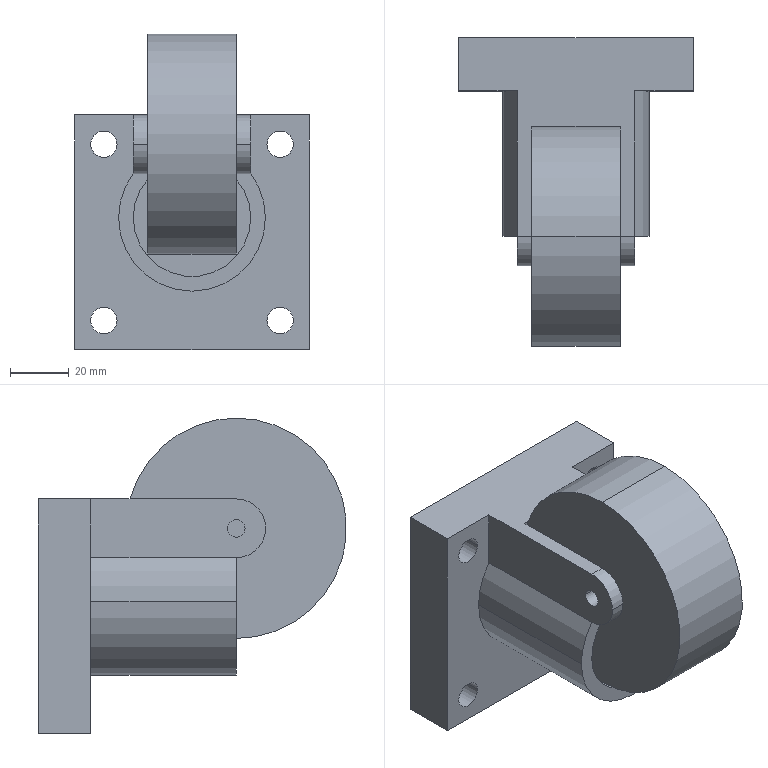Part | NX | 1 solid | 42 faces | box 80 x 105 x 107.5 mm | volume 301062 mm3 | cylinder 24 | plane 18 | commonest cylinder face diameters 9 x8 6 x4 20 x4 40 x3 50 x3 75 x2
STEP:
#1=CARTESIAN_POINT('',(-40.,4.5,0.));
#2=VERTEX_POINT('',#1);
#3=CARTESIAN_POINT('',(-40.,22.5,0.));
#4=VERTEX_POINT('',#3);
#5=CARTESIAN_POINT('',(-40.,0.,0.));
#6=DIRECTION('',(0.,1.,0.));
#7=VECTOR('',#6,1000.);
#8=LINE('',#5,#7);
#9=EDGE_CURVE('',#2,#4,#8,.T.);
#10=ORIENTED_EDGE('',*,*,#9,.T.);
#11=CARTESIAN_POINT('',(40.,22.5,0.));
#12=VERTEX_POINT('',#11);
#13=CARTESIAN_POINT('',(0.,22.5,0.));
#14=DIRECTION('',(-1.,0.,0.));
#15=VECTOR('',#14,1000.);
#16=LINE('',#13,#15);
#17=EDGE_CURVE('',#12,#4,#16,.T.);
#18=ORIENTED_EDGE('',*,*,#17,.F.);
#19=CARTESIAN_POINT('',(40.,4.5,0.));
#20=VERTEX_POINT('',#19);
#21=CARTESIAN_POINT('',(40.,0.,0.));
#22=DIRECTION('',(0.,-1.,0.));
#23=VECTOR('',#22,1000.);
#24=LINE('',#21,#23);
#25=EDGE_CURVE('',#12,#20,#24,.T.);
#26=ORIENTED_EDGE('',*,*,#25,.T.);
#27=CARTESIAN_POINT('',(0.,4.5,0.));
#28=DIRECTION('',(1.,0.,0.));
#29=VECTOR('',#28,1000.);
#30=LINE('',#27,#29);
#31=EDGE_CURVE('',#2,#20,#30,.T.);
#32=ORIENTED_EDGE('',*,*,#31,.F.);
#33=EDGE_LOOP('',(#10,#18,#26,#32));
#34=FACE_BOUND('',#33,.T.);
#35=CARTESIAN_POINT('',(0.,0.,0.));
#36=DIRECTION('',(0.,0.,1.));
#37=DIRECTION('',(1.,0.,0.));
#38=AXIS2_PLACEMENT_3D('',#35,#36,#37);
#39=PLANE('',#38);
#40=ADVANCED_FACE('',(#34),#39,.F.);
#41=ORIENTED_EDGE('',*,*,#9,.F.);
#42=CARTESIAN_POINT('',(-40.,4.5,80.));
#43=VERTEX_POINT('',#42);
#44=CARTESIAN_POINT('',(-40.,4.5,0.));
#45=DIRECTION('',(0.,0.,1.));
#46=VECTOR('',#45,1000.);
#47=LINE('',#44,#46);
#48=EDGE_CURVE('',#2,#43,#47,.T.);
#49=ORIENTED_EDGE('',*,*,#48,.T.);
#50=CARTESIAN_POINT('',(-40.,22.5,80.));
#51=VERTEX_POINT('',#50);
#52=CARTESIAN_POINT('',(-40.,0.,80.));
#53=DIRECTION('',(0.,1.,0.));
#54=VECTOR('',#53,1000.);
#55=LINE('',#52,#54);
#56=EDGE_CURVE('',#43,#51,#55,.T.);
#57=ORIENTED_EDGE('',*,*,#56,.T.);
#58=CARTESIAN_POINT('',(-40.,22.5,0.));
#59=DIRECTION('',(0.,0.,-1.));
#60=VECTOR('',#59,1000.);
#61=LINE('',#58,#60);
#62=EDGE_CURVE('',#51,#4,#61,.T.);
#63=ORIENTED_EDGE('',*,*,#62,.T.);
#64=EDGE_LOOP('',(#41,#49,#57,#63));
#65=FACE_BOUND('',#64,.T.);
#66=CARTESIAN_POINT('',(-40.,7.5,0.));
#67=DIRECTION('',(-1.,0.,0.));
#68=DIRECTION('',(0.,0.,1.));
#69=AXIS2_PLACEMENT_3D('',#66,#67,#68);
#70=PLANE('',#69);
#71=ADVANCED_FACE('',(#65),#70,.T.);
#72=ORIENTED_EDGE('',*,*,#17,.T.);
#73=ORIENTED_EDGE('',*,*,#62,.F.);
#74=CARTESIAN_POINT('',(40.,22.5,80.));
#75=VERTEX_POINT('',#74);
#76=CARTESIAN_POINT('',(0.,22.5,80.));
#77=DIRECTION('',(-1.,0.,0.));
#78=VECTOR('',#77,1000.);
#79=LINE('',#76,#78);
#80=EDGE_CURVE('',#75,#51,#79,.T.);
#81=ORIENTED_EDGE('',*,*,#80,.F.);
#82=CARTESIAN_POINT('',(40.,22.5,0.));
#83=DIRECTION('',(0.,0.,1.));
#84=VECTOR('',#83,1000.);
#85=LINE('',#82,#84);
#86=EDGE_CURVE('',#12,#75,#85,.T.);
#87=ORIENTED_EDGE('',*,*,#86,.F.);
#88=EDGE_LOOP('',(#72,#73,#81,#87));
#89=FACE_BOUND('',#88,.T.);
#90=CARTESIAN_POINT('',(25.5,22.5,10.));
#91=VERTEX_POINT('',#90);
#92=CARTESIAN_POINT('',(34.5,22.5,10.));
#93=VERTEX_POINT('',#92);
#94=CARTESIAN_POINT('',(30.,22.5,10.));
#95=DIRECTION('',(0.,-1.,0.));
#96=DIRECTION('',(1.,0.,0.));
#97=AXIS2_PLACEMENT_3D('',#94,#95,#96);
#98=CIRCLE('',#97,4.5);
#99=EDGE_CURVE('',#91,#93,#98,.T.);
#100=ORIENTED_EDGE('',*,*,#99,.T.);
#101=CARTESIAN_POINT('',(30.,22.5,10.));
#102=DIRECTION('',(0.,-1.,0.));
#103=DIRECTION('',(1.,0.,0.));
#104=AXIS2_PLACEMENT_3D('',#101,#102,#103);
#105=CIRCLE('',#104,4.5);
#106=EDGE_CURVE('',#93,#91,#105,.T.);
#107=ORIENTED_EDGE('',*,*,#106,.T.);
#108=EDGE_LOOP('',(#100,#107));
#109=FACE_BOUND('',#108,.T.);
#110=CARTESIAN_POINT('',(-34.5,22.5,10.));
#111=VERTEX_POINT('',#110);
#112=CARTESIAN_POINT('',(-25.5,22.5,10.));
#113=VERTEX_POINT('',#112);
#114=CARTESIAN_POINT('',(-30.,22.5,10.));
#115=DIRECTION('',(0.,-1.,0.));
#116=DIRECTION('',(1.,0.,0.));
#117=AXIS2_PLACEMENT_3D('',#114,#115,#116);
#118=CIRCLE('',#117,4.5);
#119=EDGE_CURVE('',#111,#113,#118,.T.);
#120=ORIENTED_EDGE('',*,*,#119,.T.);
#121=CARTESIAN_POINT('',(-30.,22.5,10.));
#122=DIRECTION('',(0.,-1.,0.));
#123=DIRECTION('',(1.,0.,0.));
#124=AXIS2_PLACEMENT_3D('',#121,#122,#123);
#125=CIRCLE('',#124,4.5);
#126=EDGE_CURVE('',#113,#111,#125,.T.);
#127=ORIENTED_EDGE('',*,*,#126,.T.);
#128=EDGE_LOOP('',(#120,#127));
#129=FACE_BOUND('',#128,.T.);
#130=CARTESIAN_POINT('',(25.5,22.5,70.));
#131=VERTEX_POINT('',#130);
#132=CARTESIAN_POINT('',(34.5,22.5,70.));
#133=VERTEX_POINT('',#132);
#134=CARTESIAN_POINT('',(30.,22.5,70.));
#135=DIRECTION('',(0.,-1.,0.));
#136=DIRECTION('',(1.,0.,0.));
#137=AXIS2_PLACEMENT_3D('',#134,#135,#136);
#138=CIRCLE('',#137,4.5);
#139=EDGE_CURVE('',#131,#133,#138,.T.);
#140=ORIENTED_EDGE('',*,*,#139,.T.);
#141=CARTESIAN_POINT('',(30.,22.5,70.));
#142=DIRECTION('',(0.,-1.,0.));
#143=DIRECTION('',(1.,0.,0.));
#144=AXIS2_PLACEMENT_3D('',#141,#142,#143);
#145=CIRCLE('',#144,4.5);
#146=EDGE_CURVE('',#133,#131,#145,.T.);
#147=ORIENTED_EDGE('',*,*,#146,.T.);
#148=EDGE_LOOP('',(#140,#147));
#149=FACE_BOUND('',#148,.T.);
#150=CARTESIAN_POINT('',(-34.5,22.5,70.));
#151=VERTEX_POINT('',#150);
#152=CARTESIAN_POINT('',(-25.5,22.5,70.));
#153=VERTEX_POINT('',#152);
#154=CARTESIAN_POINT('',(-30.,22.5,70.));
#155=DIRECTION('',(0.,-1.,0.));
#156=DIRECTION('',(1.,0.,0.));
#157=AXIS2_PLACEMENT_3D('',#154,#155,#156);
#158=CIRCLE('',#157,4.5);
#159=EDGE_CURVE('',#151,#153,#158,.T.);
#160=ORIENTED_EDGE('',*,*,#159,.T.);
#161=CARTESIAN_POINT('',(-30.,22.5,70.));
#162=DIRECTION('',(0.,-1.,0.));
#163=DIRECTION('',(1.,0.,0.));
#164=AXIS2_PLACEMENT_3D('',#161,#162,#163);
#165=CIRCLE('',#164,4.5);
#166=EDGE_CURVE('',#153,#151,#165,.T.);
#167=ORIENTED_EDGE('',*,*,#166,.T.);
#168=EDGE_LOOP('',(#160,#167));
#169=FACE_BOUND('',#168,.T.);
#170=CARTESIAN_POINT('',(40.,22.5,0.));
#171=DIRECTION('',(0.,1.,0.));
#172=DIRECTION('',(1.,0.,0.));
#173=AXIS2_PLACEMENT_3D('',#170,#171,#172);
#174=PLANE('',#173);
#175=ADVANCED_FACE('',(#89,#109,#129,#149,#169),#174,.T.);
#176=ORIENTED_EDGE('',*,*,#25,.F.);
#177=ORIENTED_EDGE('',*,*,#86,.T.);
#178=CARTESIAN_POINT('',(40.,4.5,80.));
#179=VERTEX_POINT('',#178);
#180=CARTESIAN_POINT('',(40.,0.,80.));
#181=DIRECTION('',(0.,-1.,0.));
#182=VECTOR('',#181,1000.);
#183=LINE('',#180,#182);
#184=EDGE_CURVE('',#75,#179,#183,.T.);
#185=ORIENTED_EDGE('',*,*,#184,.T.);
#186=CARTESIAN_POINT('',(40.,4.5,0.));
#187=DIRECTION('',(0.,0.,-1.));
#188=VECTOR('',#187,1000.);
#189=LINE('',#186,#188);
#190=EDGE_CURVE('',#179,#20,#189,.T.);
#191=ORIENTED_EDGE('',*,*,#190,.T.);
#192=EDGE_LOOP('',(#176,#177,#185,#191));
#193=FACE_BOUND('',#192,.T.);
#194=CARTESIAN_POINT('',(40.,-7.5,0.));
#195=DIRECTION('',(1.,0.,0.));
#196=DIRECTION('',(0.,1.,0.));
#197=AXIS2_PLACEMENT_3D('',#194,#195,#196);
#198=PLANE('',#197);
#199=ADVANCED_FACE('',(#193),#198,.T.);
#200=CARTESIAN_POINT('',(-20.,4.5,60.));
#201=VERTEX_POINT('',#200);
#202=CARTESIAN_POINT('',(-25.,4.5,45.));
#203=VERTEX_POINT('',#202);
#204=CARTESIAN_POINT('',(0.,4.5,45.));
#205=DIRECTION('',(0.,-1.,0.));
#206=DIRECTION('',(-1.,0.,0.));
#207=AXIS2_PLACEMENT_3D('',#204,#205,#206);
#208=CIRCLE('',#207,25.);
#209=EDGE_CURVE('',#201,#203,#208,.T.);
#210=ORIENTED_EDGE('',*,*,#209,.F.);
#211=CARTESIAN_POINT('',(-20.,4.5,80.));
#212=VERTEX_POINT('',#211);
#213=CARTESIAN_POINT('',(-20.,4.5,0.));
#214=DIRECTION('',(0.,0.,1.));
#215=VECTOR('',#214,1000.);
#216=LINE('',#213,#215);
#217=EDGE_CURVE('',#201,#212,#216,.T.);
#218=ORIENTED_EDGE('',*,*,#217,.T.);
#219=CARTESIAN_POINT('',(0.,4.5,80.));
#220=DIRECTION('',(1.,0.,0.));
#221=VECTOR('',#220,1000.);
#222=LINE('',#219,#221);
#223=EDGE_CURVE('',#43,#212,#222,.T.);
#224=ORIENTED_EDGE('',*,*,#223,.F.);
#225=ORIENTED_EDGE('',*,*,#48,.F.);
#226=ORIENTED_EDGE('',*,*,#31,.T.);
#227=ORIENTED_EDGE('',*,*,#190,.F.);
#228=CARTESIAN_POINT('',(20.,4.5,80.));
#229=VERTEX_POINT('',#228);
#230=CARTESIAN_POINT('',(0.,4.5,80.));
#231=DIRECTION('',(1.,0.,0.));
#232=VECTOR('',#231,1000.);
#233=LINE('',#230,#232);
#234=EDGE_CURVE('',#229,#179,#233,.T.);
#235=ORIENTED_EDGE('',*,*,#234,.F.);
#236=CARTESIAN_POINT('',(20.,4.5,60.));
#237=VERTEX_POINT('',#236);
#238=CARTESIAN_POINT('',(20.,4.5,0.));
#239=DIRECTION('',(0.,0.,-1.));
#240=VECTOR('',#239,1000.);
#241=LINE('',#238,#240);
#242=EDGE_CURVE('',#229,#237,#241,.T.);
#243=ORIENTED_EDGE('',*,*,#242,.T.);
#244=CARTESIAN_POINT('',(25.,4.5,45.));
#245=VERTEX_POINT('',#244);
#246=CARTESIAN_POINT('',(0.,4.5,45.));
#247=DIRECTION('',(0.,-1.,0.));
#248=DIRECTION('',(-1.,0.,0.));
#249=AXIS2_PLACEMENT_3D('',#246,#247,#248);
#250=CIRCLE('',#249,25.);
#251=EDGE_CURVE('',#245,#237,#250,.T.);
#252=ORIENTED_EDGE('',*,*,#251,.F.);
#253=CARTESIAN_POINT('',(0.,4.5,45.));
#254=DIRECTION('',(0.,-1.,0.));
#255=DIRECTION('',(-1.,0.,0.));
#256=AXIS2_PLACEMENT_3D('',#253,#254,#255);
#257=CIRCLE('',#256,25.);
#258=EDGE_CURVE('',#203,#245,#257,.T.);
#259=ORIENTED_EDGE('',*,*,#258,.F.);
#260=EDGE_LOOP('',(#210,#218,#224,#225,#226,#227,#235,#243,#252,#259));
#261=FACE_BOUND('',#260,.T.);
#262=CARTESIAN_POINT('',(25.5,4.5,10.));
#263=VERTEX_POINT('',#262);
#264=CARTESIAN_POINT('',(34.5,4.5,10.));
#265=VERTEX_POINT('',#264);
#266=CARTESIAN_POINT('',(30.,4.5,10.));
#267=DIRECTION('',(0.,-1.,0.));
#268=DIRECTION('',(1.,0.,0.));
#269=AXIS2_PLACEMENT_3D('',#266,#267,#268);
#270=CIRCLE('',#269,4.5);
#271=EDGE_CURVE('',#263,#265,#270,.T.);
#272=ORIENTED_EDGE('',*,*,#271,.F.);
#273=CARTESIAN_POINT('',(30.,4.5,10.));
#274=DIRECTION('',(0.,-1.,0.));
#275=DIRECTION('',(1.,0.,0.));
#276=AXIS2_PLACEMENT_3D('',#273,#274,#275);
#277=CIRCLE('',#276,4.5);
#278=EDGE_CURVE('',#265,#263,#277,.T.);
#279=ORIENTED_EDGE('',*,*,#278,.F.);
#280=EDGE_LOOP('',(#272,#279));
#281=FACE_BOUND('',#280,.T.);
#282=CARTESIAN_POINT('',(-34.5,4.5,10.));
#283=VERTEX_POINT('',#282);
#284=CARTESIAN_POINT('',(-25.5,4.5,10.));
#285=VERTEX_POINT('',#284);
#286=CARTESIAN_POINT('',(-30.,4.5,10.));
#287=DIRECTION('',(0.,-1.,0.));
#288=DIRECTION('',(1.,0.,0.));
#289=AXIS2_PLACEMENT_3D('',#286,#287,#288);
#290=CIRCLE('',#289,4.5);
#291=EDGE_CURVE('',#283,#285,#290,.T.);
#292=ORIENTED_EDGE('',*,*,#291,.F.);
#293=CARTESIAN_POINT('',(-30.,4.5,10.));
#294=DIRECTION('',(0.,-1.,0.));
#295=DIRECTION('',(1.,0.,0.));
#296=AXIS2_PLACEMENT_3D('',#293,#294,#295);
#297=CIRCLE('',#296,4.5);
#298=EDGE_CURVE('',#285,#283,#297,.T.);
#299=ORIENTED_EDGE('',*,*,#298,.F.);
#300=EDGE_LOOP('',(#292,#299));
#301=FACE_BOUND('',#300,.T.);
#302=CARTESIAN_POINT('',(25.5,4.5,70.));
#303=VERTEX_POINT('',#302);
#304=CARTESIAN_POINT('',(34.5,4.5,70.));
#305=VERTEX_POINT('',#304);
#306=CARTESIAN_POINT('',(30.,4.5,70.));
#307=DIRECTION('',(0.,-1.,0.));
#308=DIRECTION('',(1.,0.,0.));
#309=AXIS2_PLACEMENT_3D('',#306,#307,#308);
#310=CIRCLE('',#309,4.5);
#311=EDGE_CURVE('',#303,#305,#310,.T.);
#312=ORIENTED_EDGE('',*,*,#311,.F.);
#313=CARTESIAN_POINT('',(30.,4.5,70.));
#314=DIRECTION('',(0.,-1.,0.));
#315=DIRECTION('',(1.,0.,0.));
#316=AXIS2_PLACEMENT_3D('',#313,#314,#315);
#317=CIRCLE('',#316,4.5);
#318=EDGE_CURVE('',#305,#303,#317,.T.);
#319=ORIENTED_EDGE('',*,*,#318,.F.);
#320=EDGE_LOOP('',(#312,#319));
#321=FACE_BOUND('',#320,.T.);
#322=CARTESIAN_POINT('',(-34.5,4.5,70.));
#323=VERTEX_POINT('',#322);
#324=CARTESIAN_POINT('',(-25.5,4.5,70.));
#325=VERTEX_POINT('',#324);
#326=CARTESIAN_POINT('',(-30.,4.5,70.));
#327=DIRECTION('',(0.,-1.,0.));
#328=DIRECTION('',(1.,0.,0.));
#329=AXIS2_PLACEMENT_3D('',#326,#327,#328);
#330=CIRCLE('',#329,4.5);
#331=EDGE_CURVE('',#323,#325,#330,.T.);
#332=ORIENTED_EDGE('',*,*,#331,.F.);
#333=CARTESIAN_POINT('',(-30.,4.5,70.));
#334=DIRECTION('',(0.,-1.,0.));
#335=DIRECTION('',(1.,0.,0.));
#336=AXIS2_PLACEMENT_3D('',#333,#334,#335);
#337=CIRCLE('',#336,4.5);
#338=EDGE_CURVE('',#325,#323,#337,.T.);
#339=ORIENTED_EDGE('',*,*,#338,.F.);
#340=EDGE_LOOP('',(#332,#339));
#341=FACE_BOUND('',#340,.T.);
#342=CARTESIAN_POINT('',(-40.,4.5,0.));
#343=DIRECTION('',(0.,-1.,0.));
#344=DIRECTION('',(0.,0.,-1.));
#345=AXIS2_PLACEMENT_3D('',#342,#343,#344);
#346=PLANE('',#345);
#347=ADVANCED_FACE('',(#261,#281,#301,#321,#341),#346,.T.);
#348=CARTESIAN_POINT('',(25.,-45.,45.));
#349=VERTEX_POINT('',#348);
#350=CARTESIAN_POINT('',(25.,-7.5,45.));
#351=DIRECTION('',(0.,-1.,0.));
#352=VECTOR('',#351,1000.);
#353=LINE('',#350,#352);
#354=EDGE_CURVE('',#245,#349,#353,.T.);
#355=ORIENTED_EDGE('',*,*,#354,.F.);
#356=ORIENTED_EDGE('',*,*,#251,.T.);
#357=CARTESIAN_POINT('',(20.,-45.,60.));
#358=VERTEX_POINT('',#357);
#359=CARTESIAN_POINT('',(20.,-7.5,60.));
#360=DIRECTION('',(0.,1.,0.));
#361=VECTOR('',#360,1000.);
#362=LINE('',#359,#361);
#363=EDGE_CURVE('',#358,#237,#362,.T.);
#364=ORIENTED_EDGE('',*,*,#363,.F.);
#365=CARTESIAN_POINT('',(0.,-45.,45.));
#366=DIRECTION('',(0.,1.,0.));
#367=DIRECTION('',(0.8,0.,0.6));
#368=AXIS2_PLACEMENT_3D('',#365,#366,#367);
#369=CIRCLE('',#368,25.);
#370=EDGE_CURVE('',#358,#349,#369,.T.);
#371=ORIENTED_EDGE('',*,*,#370,.T.);
#372=EDGE_LOOP('',(#355,#356,#364,#371));
#373=FACE_BOUND('',#372,.T.);
#374=CARTESIAN_POINT('',(0.,-7.5,45.));
#375=DIRECTION('',(0.,-1.,0.));
#376=DIRECTION('',(-1.,0.,0.));
#377=AXIS2_PLACEMENT_3D('',#374,#375,#376);
#378=CYLINDRICAL_SURFACE('',#377,25.);
#379=ADVANCED_FACE('',(#373),#378,.T.);
#380=CARTESIAN_POINT('',(15.,-45.,58.229));
#381=VERTEX_POINT('',#380);
#382=CARTESIAN_POINT('',(15.,-45.,60.));
#383=VERTEX_POINT('',#382);
#384=CARTESIAN_POINT('',(15.,-45.,58.229));
#385=DIRECTION('',(0.,0.,1.));
#386=VECTOR('',#385,1000.);
#387=LINE('',#384,#386);
#388=EDGE_CURVE('',#381,#383,#387,.T.);
#389=ORIENTED_EDGE('',*,*,#388,.F.);
#390=CARTESIAN_POINT('',(20.,-45.,45.));
#391=VERTEX_POINT('',#390);
#392=CARTESIAN_POINT('',(0.,-45.,45.));
#393=DIRECTION('',(0.,-1.,0.));
#394=DIRECTION('',(1.,0.,0.));
#395=AXIS2_PLACEMENT_3D('',#392,#393,#394);
#396=CIRCLE('',#395,20.);
#397=EDGE_CURVE('',#391,#381,#396,.T.);
#398=ORIENTED_EDGE('',*,*,#397,.F.);
#399=CARTESIAN_POINT('',(-20.,-45.,45.));
#400=VERTEX_POINT('',#399);
#401=CARTESIAN_POINT('',(0.,-45.,45.));
#402=DIRECTION('',(0.,-1.,0.));
#403=DIRECTION('',(1.,0.,0.));
#404=AXIS2_PLACEMENT_3D('',#401,#402,#403);
#405=CIRCLE('',#404,20.);
#406=EDGE_CURVE('',#400,#391,#405,.T.);
#407=ORIENTED_EDGE('',*,*,#406,.F.);
#408=CARTESIAN_POINT('',(-15.,-45.,58.229));
#409=VERTEX_POINT('',#408);
#410=CARTESIAN_POINT('',(0.,-45.,45.));
#411=DIRECTION('',(0.,-1.,0.));
#412=DIRECTION('',(1.,0.,0.));
#413=AXIS2_PLACEMENT_3D('',#410,#411,#412);
#414=CIRCLE('',#413,20.);
#415=EDGE_CURVE('',#409,#400,#414,.T.);
#416=ORIENTED_EDGE('',*,*,#415,.F.);
#417=CARTESIAN_POINT('',(-15.,-45.,60.));
#418=VERTEX_POINT('',#417);
#419=CARTESIAN_POINT('',(-15.,-45.,58.229));
#420=DIRECTION('',(0.,0.,1.));
#421=VECTOR('',#420,1000.);
#422=LINE('',#419,#421);
#423=EDGE_CURVE('',#409,#418,#422,.T.);
#424=ORIENTED_EDGE('',*,*,#423,.T.);
#425=CARTESIAN_POINT('',(-20.,-45.,60.));
#426=VERTEX_POINT('',#425);
#427=CARTESIAN_POINT('',(-15.,-45.,60.));
#428=DIRECTION('',(-1.,0.,0.));
#429=VECTOR('',#428,1000.);
#430=LINE('',#427,#429);
#431=EDGE_CURVE('',#418,#426,#430,.T.);
#432=ORIENTED_EDGE('',*,*,#431,.T.);
#433=CARTESIAN_POINT('',(-25.,-45.,45.));
#434=VERTEX_POINT('',#433);
#435=CARTESIAN_POINT('',(0.,-45.,45.));
#436=DIRECTION('',(0.,1.,0.));
#437=DIRECTION('',(0.8,0.,0.6));
#438=AXIS2_PLACEMENT_3D('',#435,#436,#437);
#439=CIRCLE('',#438,25.);
#440=EDGE_CURVE('',#434,#426,#439,.T.);
#441=ORIENTED_EDGE('',*,*,#440,.F.);
#442=CARTESIAN_POINT('',(0.,-45.,45.));
#443=DIRECTION('',(0.,1.,0.));
#444=DIRECTION('',(0.8,0.,0.6));
#445=AXIS2_PLACEMENT_3D('',#442,#443,#444);
#446=CIRCLE('',#445,25.);
#447=EDGE_CURVE('',#349,#434,#446,.T.);
#448=ORIENTED_EDGE('',*,*,#447,.F.);
#449=ORIENTED_EDGE('',*,*,#370,.F.);
#450=CARTESIAN_POINT('',(20.,-45.,60.));
#451=DIRECTION('',(-1.,0.,0.));
#452=VECTOR('',#451,1000.);
#453=LINE('',#450,#452);
#454=EDGE_CURVE('',#358,#383,#453,.T.);
#455=ORIENTED_EDGE('',*,*,#454,.T.);
#456=EDGE_LOOP('',(#389,#398,#407,#416,#424,#432,#441,#448,#449,#455));
#457=FACE_BOUND('',#456,.T.);
#458=CARTESIAN_POINT('',(25.,-45.,20.));
#459=DIRECTION('',(0.,1.,0.));
#460=DIRECTION('',(1.,0.,0.));
#461=AXIS2_PLACEMENT_3D('',#458,#459,#460);
#462=PLANE('',#461);
#463=ADVANCED_FACE('',(#457),#462,.F.);
#464=CARTESIAN_POINT('',(15.,-8.858,80.));
#465=VERTEX_POINT('',#464);
#466=CARTESIAN_POINT('',(15.,-45.,80.));
#467=VERTEX_POINT('',#466);
#468=CARTESIAN_POINT('',(15.,-8.858,80.));
#469=DIRECTION('',(0.,-1.,0.));
#470=VECTOR('',#469,1000.);
#471=LINE('',#468,#470);
#472=EDGE_CURVE('',#465,#467,#471,.T.);
#473=ORIENTED_EDGE('',*,*,#472,.F.);
#474=CARTESIAN_POINT('',(15.,-45.,107.5));
#475=VERTEX_POINT('',#474);
#476=CARTESIAN_POINT('',(15.,-45.,70.));
#477=DIRECTION('',(-1.,0.,0.));
#478=DIRECTION('',(0.,0.,1.));
#479=AXIS2_PLACEMENT_3D('',#476,#477,#478);
#480=CIRCLE('',#479,37.5);
#481=EDGE_CURVE('',#475,#465,#480,.T.);
#482=ORIENTED_EDGE('',*,*,#481,.F.);
#483=CARTESIAN_POINT('',(15.,-45.,32.5));
#484=VERTEX_POINT('',#483);
#485=CARTESIAN_POINT('',(15.,-45.,70.));
#486=DIRECTION('',(-1.,0.,0.));
#487=DIRECTION('',(0.,0.,1.));
#488=AXIS2_PLACEMENT_3D('',#485,#486,#487);
#489=CIRCLE('',#488,37.5);
#490=EDGE_CURVE('',#484,#475,#489,.T.);
#491=ORIENTED_EDGE('',*,*,#490,.F.);
#492=CARTESIAN_POINT('',(15.,-9.395,58.229));
#493=VERTEX_POINT('',#492);
#494=CARTESIAN_POINT('',(15.,-45.,70.));
#495=DIRECTION('',(-1.,0.,0.));
#496=DIRECTION('',(0.,0.,1.));
#497=AXIS2_PLACEMENT_3D('',#494,#495,#496);
#498=CIRCLE('',#497,37.5);
#499=EDGE_CURVE('',#493,#484,#498,.T.);
#500=ORIENTED_EDGE('',*,*,#499,.F.);
#501=CARTESIAN_POINT('',(15.,-9.395,58.229));
#502=DIRECTION('',(0.,-1.,0.));
#503=VECTOR('',#502,1000.);
#504=LINE('',#501,#503);
#505=EDGE_CURVE('',#493,#381,#504,.T.);
#506=ORIENTED_EDGE('',*,*,#505,.T.);
#507=ORIENTED_EDGE('',*,*,#388,.T.);
#508=CARTESIAN_POINT('',(15.,-55.,70.));
#509=VERTEX_POINT('',#508);
#510=CARTESIAN_POINT('',(15.,-45.,70.));
#511=DIRECTION('',(1.,0.,0.));
#512=DIRECTION('',(0.,-1.,0.));
#513=AXIS2_PLACEMENT_3D('',#510,#511,#512);
#514=CIRCLE('',#513,10.);
#515=EDGE_CURVE('',#509,#383,#514,.T.);
#516=ORIENTED_EDGE('',*,*,#515,.F.);
#517=CARTESIAN_POINT('',(15.,-45.,70.));
#518=DIRECTION('',(1.,0.,0.));
#519=DIRECTION('',(0.,-1.,0.));
#520=AXIS2_PLACEMENT_3D('',#517,#518,#519);
#521=CIRCLE('',#520,10.);
#522=EDGE_CURVE('',#467,#509,#521,.T.);
#523=ORIENTED_EDGE('',*,*,#522,.F.);
#524=EDGE_LOOP('',(#473,#482,#491,#500,#506,#507,#516,#523));
#525=FACE_BOUND('',#524,.T.);
#526=CARTESIAN_POINT('',(15.,7.5,0.));
#527=DIRECTION('',(-1.,0.,0.));
#528=DIRECTION('',(0.,0.,1.));
#529=AXIS2_PLACEMENT_3D('',#526,#527,#528);
#530=PLANE('',#529);
#531=ADVANCED_FACE('',(#525),#530,.F.);
#532=ORIENTED_EDGE('',*,*,#472,.T.);
#533=CARTESIAN_POINT('',(20.,-45.,80.));
#534=VERTEX_POINT('',#533);
#535=CARTESIAN_POINT('',(15.,-45.,80.));
#536=DIRECTION('',(1.,0.,0.));
#537=VECTOR('',#536,1000.);
#538=LINE('',#535,#537);
#539=EDGE_CURVE('',#467,#534,#538,.T.);
#540=ORIENTED_EDGE('',*,*,#539,.T.);
#541=CARTESIAN_POINT('',(20.,0.,80.));
#542=DIRECTION('',(0.,1.,0.));
#543=VECTOR('',#542,1000.);
#544=LINE('',#541,#543);
#545=EDGE_CURVE('',#534,#229,#544,.T.);
#546=ORIENTED_EDGE('',*,*,#545,.T.);
#547=ORIENTED_EDGE('',*,*,#234,.T.);
#548=ORIENTED_EDGE('',*,*,#184,.F.);
#549=ORIENTED_EDGE('',*,*,#80,.T.);
#550=ORIENTED_EDGE('',*,*,#56,.F.);
#551=ORIENTED_EDGE('',*,*,#223,.T.);
#552=CARTESIAN_POINT('',(-20.,-45.,80.));
#553=VERTEX_POINT('',#552);
#554=CARTESIAN_POINT('',(-20.,0.,80.));
#555=DIRECTION('',(0.,1.,0.));
#556=VECTOR('',#555,1000.);
#557=LINE('',#554,#556);
#558=EDGE_CURVE('',#553,#212,#557,.T.);
#559=ORIENTED_EDGE('',*,*,#558,.F.);
#560=CARTESIAN_POINT('',(-15.,-45.,80.));
#561=VERTEX_POINT('',#560);
#562=CARTESIAN_POINT('',(-20.,-45.,80.));
#563=DIRECTION('',(1.,0.,0.));
#564=VECTOR('',#563,1000.);
#565=LINE('',#562,#564);
#566=EDGE_CURVE('',#553,#561,#565,.T.);
#567=ORIENTED_EDGE('',*,*,#566,.T.);
#568=CARTESIAN_POINT('',(-15.,-8.858,80.));
#569=VERTEX_POINT('',#568);
#570=CARTESIAN_POINT('',(-15.,-45.,80.));
#571=DIRECTION('',(0.,1.,0.));
#572=VECTOR('',#571,1000.);
#573=LINE('',#570,#572);
#574=EDGE_CURVE('',#561,#569,#573,.T.);
#575=ORIENTED_EDGE('',*,*,#574,.T.);
#576=CARTESIAN_POINT('',(-15.,-7.5,80.));
#577=VERTEX_POINT('',#576);
#578=CARTESIAN_POINT('',(-15.,-7.5,80.));
#579=DIRECTION('',(0.,-1.,0.));
#580=VECTOR('',#579,1000.);
#581=LINE('',#578,#580);
#582=EDGE_CURVE('',#577,#569,#581,.T.);
#583=ORIENTED_EDGE('',*,*,#582,.F.);
#584=CARTESIAN_POINT('',(15.,-7.5,80.));
#585=VERTEX_POINT('',#584);
#586=CARTESIAN_POINT('',(-15.,-7.5,80.));
#587=DIRECTION('',(1.,0.,0.));
#588=VECTOR('',#587,1000.);
#589=LINE('',#586,#588);
#590=EDGE_CURVE('',#577,#585,#589,.T.);
#591=ORIENTED_EDGE('',*,*,#590,.T.);
#592=CARTESIAN_POINT('',(15.,-7.5,80.));
#593=DIRECTION('',(0.,-1.,0.));
#594=VECTOR('',#593,1000.);
#595=LINE('',#592,#594);
#596=EDGE_CURVE('',#585,#465,#595,.T.);
#597=ORIENTED_EDGE('',*,*,#596,.T.);
#598=EDGE_LOOP('',(#532,#540,#546,#547,#548,#549,#550,#551,#559,#567,#575,#583,#591,#597));
#599=FACE_BOUND('',#598,.T.);
#600=CARTESIAN_POINT('',(0.,0.,80.));
#601=DIRECTION('',(0.,0.,1.));
#602=DIRECTION('',(1.,0.,0.));
#603=AXIS2_PLACEMENT_3D('',#600,#601,#602);
#604=PLANE('',#603);
#605=ADVANCED_FACE('',(#599),#604,.T.);
#606=CARTESIAN_POINT('',(15.,-7.5,70.));
#607=VERTEX_POINT('',#606);
#608=CARTESIAN_POINT('',(15.,-45.,70.));
#609=DIRECTION('',(-1.,0.,0.));
#610=DIRECTION('',(0.,0.9638,0.2667));
#611=AXIS2_PLACEMENT_3D('',#608,#609,#610);
#612=CIRCLE('',#611,37.5);
#613=EDGE_CURVE('',#465,#607,#612,.T.);
#614=ORIENTED_EDGE('',*,*,#613,.F.);
#615=ORIENTED_EDGE('',*,*,#596,.F.);
#616=CARTESIAN_POINT('',(15.,-7.5,80.));
#617=DIRECTION('',(0.,0.,-1.));
#618=VECTOR('',#617,1000.);
#619=LINE('',#616,#618);
#620=EDGE_CURVE('',#585,#607,#619,.T.);
#621=ORIENTED_EDGE('',*,*,#620,.T.);
#622=EDGE_LOOP('',(#614,#615,#621));
#623=FACE_BOUND('',#622,.T.);
#624=CARTESIAN_POINT('',(15.,-55.,58.229));
#625=DIRECTION('',(1.,0.,0.));
#626=DIRECTION('',(0.,1.,0.));
#627=AXIS2_PLACEMENT_3D('',#624,#625,#626);
#628=PLANE('',#627);
#629=ADVANCED_FACE('',(#623),#628,.F.);
#630=CARTESIAN_POINT('',(-15.,-45.,32.5));
#631=VERTEX_POINT('',#630);
#632=CARTESIAN_POINT('',(-15.,-9.395,58.229));
#633=VERTEX_POINT('',#632);
#634=CARTESIAN_POINT('',(-15.,-45.,70.));
#635=DIRECTION('',(1.,0.,0.));
#636=DIRECTION('',(0.,0.9638,0.2667));
#637=AXIS2_PLACEMENT_3D('',#634,#635,#636);
#638=CIRCLE('',#637,37.5);
#639=EDGE_CURVE('',#631,#633,#638,.T.);
#640=ORIENTED_EDGE('',*,*,#639,.T.);
#641=CARTESIAN_POINT('',(-15.,-7.5,70.));
#642=VERTEX_POINT('',#641);
#643=CARTESIAN_POINT('',(-15.,-45.,70.));
#644=DIRECTION('',(1.,0.,0.));
#645=DIRECTION('',(0.,0.9495,-0.3139));
#646=AXIS2_PLACEMENT_3D('',#643,#644,#645);
#647=CIRCLE('',#646,37.5);
#648=EDGE_CURVE('',#633,#642,#647,.T.);
#649=ORIENTED_EDGE('',*,*,#648,.T.);
#650=CARTESIAN_POINT('',(-15.,-45.,70.));
#651=DIRECTION('',(1.,0.,0.));
#652=DIRECTION('',(0.,1.,0.));
#653=AXIS2_PLACEMENT_3D('',#650,#651,#652);
#654=CIRCLE('',#653,37.5);
#655=EDGE_CURVE('',#642,#569,#654,.T.);
#656=ORIENTED_EDGE('',*,*,#655,.T.);
#657=CARTESIAN_POINT('',(-15.,-45.,107.5));
#658=VERTEX_POINT('',#657);
#659=CARTESIAN_POINT('',(-15.,-45.,70.));
#660=DIRECTION('',(1.,0.,0.));
#661=DIRECTION('',(0.,0.9638,0.2667));
#662=AXIS2_PLACEMENT_3D('',#659,#660,#661);
#663=CIRCLE('',#662,37.5);
#664=EDGE_CURVE('',#569,#658,#663,.T.);
#665=ORIENTED_EDGE('',*,*,#664,.T.);
#666=CARTESIAN_POINT('',(15.,-45.,107.5));
#667=DIRECTION('',(-1.,0.,0.));
#668=VECTOR('',#667,1000.);
#669=LINE('',#666,#668);
#670=EDGE_CURVE('',#475,#658,#669,.T.);
#671=ORIENTED_EDGE('',*,*,#670,.F.);
#672=ORIENTED_EDGE('',*,*,#481,.T.);
#673=ORIENTED_EDGE('',*,*,#613,.T.);
#674=CARTESIAN_POINT('',(15.,-45.,70.));
#675=DIRECTION('',(-1.,0.,0.));
#676=DIRECTION('',(0.,1.,0.));
#677=AXIS2_PLACEMENT_3D('',#674,#675,#676);
#678=CIRCLE('',#677,37.5);
#679=EDGE_CURVE('',#607,#493,#678,.T.);
#680=ORIENTED_EDGE('',*,*,#679,.T.);
#681=ORIENTED_EDGE('',*,*,#499,.T.);
#682=CARTESIAN_POINT('',(15.,-45.,32.5));
#683=DIRECTION('',(-1.,0.,0.));
#684=VECTOR('',#683,1000.);
#685=LINE('',#682,#684);
#686=EDGE_CURVE('',#484,#631,#685,.T.);
#687=ORIENTED_EDGE('',*,*,#686,.T.);
#688=EDGE_LOOP('',(#640,#649,#656,#665,#671,#672,#673,#680,#681,#687));
#689=FACE_BOUND('',#688,.T.);
#690=CARTESIAN_POINT('',(15.,-45.,70.));
#691=DIRECTION('',(-1.,0.,0.));
#692=DIRECTION('',(0.,0.,1.));
#693=AXIS2_PLACEMENT_3D('',#690,#691,#692);
#694=CYLINDRICAL_SURFACE('',#693,37.5);
#695=ADVANCED_FACE('',(#689),#694,.T.);
#696=ORIENTED_EDGE('',*,*,#119,.F.);
#697=CARTESIAN_POINT('',(-34.5,7.5,10.));
#698=DIRECTION('',(0.,-1.,0.));
#699=VECTOR('',#698,1000.);
#700=LINE('',#697,#699);
#701=EDGE_CURVE('',#111,#283,#700,.T.);
#702=ORIENTED_EDGE('',*,*,#701,.T.);
#703=ORIENTED_EDGE('',*,*,#291,.T.);
#704=CARTESIAN_POINT('',(-25.5,7.5,10.));
#705=DIRECTION('',(0.,-1.,0.));
#706=VECTOR('',#705,1000.);
#707=LINE('',#704,#706);
#708=EDGE_CURVE('',#113,#285,#707,.T.);
#709=ORIENTED_EDGE('',*,*,#708,.F.);
#710=EDGE_LOOP('',(#696,#702,#703,#709));
#711=FACE_BOUND('',#710,.T.);
#712=CARTESIAN_POINT('',(-30.,7.5,10.));
#713=DIRECTION('',(0.,-1.,0.));
#714=DIRECTION('',(1.,0.,0.));
#715=AXIS2_PLACEMENT_3D('',#712,#713,#714);
#716=CYLINDRICAL_SURFACE('',#715,4.5);
#717=ADVANCED_FACE('',(#711),#716,.F.);
#718=ORIENTED_EDGE('',*,*,#574,.F.);
#719=CARTESIAN_POINT('',(-15.,-55.,70.));
#720=VERTEX_POINT('',#719);
#721=CARTESIAN_POINT('',(-15.,-45.,70.));
#722=DIRECTION('',(-1.,0.,0.));
#723=DIRECTION('',(0.,-1.,0.));
#724=AXIS2_PLACEMENT_3D('',#721,#722,#723);
#725=CIRCLE('',#724,10.);
#726=EDGE_CURVE('',#720,#561,#725,.T.);
#727=ORIENTED_EDGE('',*,*,#726,.F.);
#728=CARTESIAN_POINT('',(-15.,-45.,70.));
#729=DIRECTION('',(-1.,0.,0.));
#730=DIRECTION('',(0.,-1.,0.));
#731=AXIS2_PLACEMENT_3D('',#728,#729,#730);
#732=CIRCLE('',#731,10.);
#733=EDGE_CURVE('',#418,#720,#732,.T.);
#734=ORIENTED_EDGE('',*,*,#733,.F.);
#735=ORIENTED_EDGE('',*,*,#423,.F.);
#736=CARTESIAN_POINT('',(-15.,-45.,58.229));
#737=DIRECTION('',(0.,1.,0.));
#738=VECTOR('',#737,1000.);
#739=LINE('',#736,#738);
#740=EDGE_CURVE('',#409,#633,#739,.T.);
#741=ORIENTED_EDGE('',*,*,#740,.T.);
#742=ORIENTED_EDGE('',*,*,#639,.F.);
#743=CARTESIAN_POINT('',(-15.,-45.,70.));
#744=DIRECTION('',(1.,0.,0.));
#745=DIRECTION('',(0.,0.9638,0.2667));
#746=AXIS2_PLACEMENT_3D('',#743,#744,#745);
#747=CIRCLE('',#746,37.5);
#748=EDGE_CURVE('',#658,#631,#747,.T.);
#749=ORIENTED_EDGE('',*,*,#748,.F.);
#750=ORIENTED_EDGE('',*,*,#664,.F.);
#751=EDGE_LOOP('',(#718,#727,#734,#735,#741,#742,#749,#750));
#752=FACE_BOUND('',#751,.T.);
#753=CARTESIAN_POINT('',(-15.,7.5,0.));
#754=DIRECTION('',(-1.,0.,0.));
#755=DIRECTION('',(0.,0.,1.));
#756=AXIS2_PLACEMENT_3D('',#753,#754,#755);
#757=PLANE('',#756);
#758=ADVANCED_FACE('',(#752),#757,.T.);
#759=CARTESIAN_POINT('',(-20.,-7.5,45.));
#760=VERTEX_POINT('',#759);
#761=CARTESIAN_POINT('',(-20.,-55.,45.));
#762=DIRECTION('',(0.,-1.,0.));
#763=VECTOR('',#762,1000.);
#764=LINE('',#761,#763);
#765=EDGE_CURVE('',#760,#400,#764,.T.);
#766=ORIENTED_EDGE('',*,*,#765,.F.);
#767=CARTESIAN_POINT('',(-15.,-7.5,58.229));
#768=VERTEX_POINT('',#767);
#769=CARTESIAN_POINT('',(0.,-7.5,45.));
#770=DIRECTION('',(0.,1.,0.));
#771=DIRECTION('',(0.75,0.,0.6614));
#772=AXIS2_PLACEMENT_3D('',#769,#770,#771);
#773=CIRCLE('',#772,20.);
#774=EDGE_CURVE('',#760,#768,#773,.T.);
#775=ORIENTED_EDGE('',*,*,#774,.T.);
#776=CARTESIAN_POINT('',(-15.,-9.395,58.229));
#777=DIRECTION('',(0.,1.,0.));
#778=VECTOR('',#777,1000.);
#779=LINE('',#776,#778);
#780=EDGE_CURVE('',#633,#768,#779,.T.);
#781=ORIENTED_EDGE('',*,*,#780,.F.);
#782=ORIENTED_EDGE('',*,*,#740,.F.);
#783=ORIENTED_EDGE('',*,*,#415,.T.);
#784=EDGE_LOOP('',(#766,#775,#781,#782,#783));
#785=FACE_BOUND('',#784,.T.);
#786=CARTESIAN_POINT('',(0.,-55.,45.));
#787=DIRECTION('',(0.,-1.,0.));
#788=DIRECTION('',(-1.,0.,0.));
#789=AXIS2_PLACEMENT_3D('',#786,#787,#788);
#790=CYLINDRICAL_SURFACE('',#789,20.);
#791=ADVANCED_FACE('',(#785),#790,.F.);
#792=ORIENTED_EDGE('',*,*,#780,.T.);
#793=CARTESIAN_POINT('',(-15.,-7.5,58.229));
#794=DIRECTION('',(0.,0.,1.));
#795=VECTOR('',#794,1000.);
#796=LINE('',#793,#795);
#797=EDGE_CURVE('',#768,#642,#796,.T.);
#798=ORIENTED_EDGE('',*,*,#797,.T.);
#799=ORIENTED_EDGE('',*,*,#648,.F.);
#800=EDGE_LOOP('',(#792,#798,#799));
#801=FACE_BOUND('',#800,.T.);
#802=CARTESIAN_POINT('',(-15.,-55.,80.));
#803=DIRECTION('',(-1.,0.,0.));
#804=DIRECTION('',(0.,0.,1.));
#805=AXIS2_PLACEMENT_3D('',#802,#803,#804);
#806=PLANE('',#805);
#807=ADVANCED_FACE('',(#801),#806,.F.);
#808=CARTESIAN_POINT('',(15.,-7.5,58.229));
#809=VERTEX_POINT('',#808);
#810=CARTESIAN_POINT('',(15.,-7.5,70.));
#811=DIRECTION('',(0.,0.,-1.));
#812=VECTOR('',#811,1000.);
#813=LINE('',#810,#812);
#814=EDGE_CURVE('',#607,#809,#813,.T.);
#815=ORIENTED_EDGE('',*,*,#814,.F.);
#816=ORIENTED_EDGE('',*,*,#620,.F.);
#817=ORIENTED_EDGE('',*,*,#590,.F.);
#818=CARTESIAN_POINT('',(-15.,-7.5,70.));
#819=DIRECTION('',(0.,0.,1.));
#820=VECTOR('',#819,1000.);
#821=LINE('',#818,#820);
#822=EDGE_CURVE('',#642,#577,#821,.T.);
#823=ORIENTED_EDGE('',*,*,#822,.F.);
#824=ORIENTED_EDGE('',*,*,#797,.F.);
#825=ORIENTED_EDGE('',*,*,#774,.F.);
#826=CARTESIAN_POINT('',(20.,-7.5,45.));
#827=VERTEX_POINT('',#826);
#828=CARTESIAN_POINT('',(0.,-7.5,45.));
#829=DIRECTION('',(0.,1.,0.));
#830=DIRECTION('',(0.75,0.,0.6614));
#831=AXIS2_PLACEMENT_3D('',#828,#829,#830);
#832=CIRCLE('',#831,20.);
#833=EDGE_CURVE('',#827,#760,#832,.T.);
#834=ORIENTED_EDGE('',*,*,#833,.F.);
#835=CARTESIAN_POINT('',(0.,-7.5,45.));
#836=DIRECTION('',(0.,1.,0.));
#837=DIRECTION('',(0.75,0.,0.6614));
#838=AXIS2_PLACEMENT_3D('',#835,#836,#837);
#839=CIRCLE('',#838,20.);
#840=EDGE_CURVE('',#809,#827,#839,.T.);
#841=ORIENTED_EDGE('',*,*,#840,.F.);
#842=EDGE_LOOP('',(#815,#816,#817,#823,#824,#825,#834,#841));
#843=FACE_BOUND('',#842,.T.);
#844=CARTESIAN_POINT('',(0.,-7.5,0.));
#845=DIRECTION('',(0.,-1.,0.));
#846=DIRECTION('',(0.,0.,-1.));
#847=AXIS2_PLACEMENT_3D('',#844,#845,#846);
#848=PLANE('',#847);
#849=ADVANCED_FACE('',(#843),#848,.T.);
#850=CARTESIAN_POINT('',(15.,-7.5,58.229));
#851=DIRECTION('',(0.,-1.,0.));
#852=VECTOR('',#851,1000.);
#853=LINE('',#850,#852);
#854=EDGE_CURVE('',#809,#493,#853,.T.);
#855=ORIENTED_EDGE('',*,*,#854,.T.);
#856=ORIENTED_EDGE('',*,*,#679,.F.);
#857=ORIENTED_EDGE('',*,*,#814,.T.);
#858=EDGE_LOOP('',(#855,#856,#857));
#859=FACE_BOUND('',#858,.T.);
#860=CARTESIAN_POINT('',(15.,-55.,58.229));
#861=DIRECTION('',(1.,0.,0.));
#862=DIRECTION('',(0.,1.,0.));
#863=AXIS2_PLACEMENT_3D('',#860,#861,#862);
#864=PLANE('',#863);
#865=ADVANCED_FACE('',(#859),#864,.F.);
#866=ORIENTED_EDGE('',*,*,#655,.F.);
#867=ORIENTED_EDGE('',*,*,#822,.T.);
#868=ORIENTED_EDGE('',*,*,#582,.T.);
#869=EDGE_LOOP('',(#866,#867,#868));
#870=FACE_BOUND('',#869,.T.);
#871=CARTESIAN_POINT('',(-15.,-55.,80.));
#872=DIRECTION('',(-1.,0.,0.));
#873=DIRECTION('',(0.,0.,1.));
#874=AXIS2_PLACEMENT_3D('',#871,#872,#873);
#875=PLANE('',#874);
#876=ADVANCED_FACE('',(#870),#875,.F.);
#877=CARTESIAN_POINT('',(-20.,-55.,70.));
#878=VERTEX_POINT('',#877);
#879=CARTESIAN_POINT('',(-20.173,-55.,70.));
#880=DIRECTION('',(1.,0.,0.));
#881=VECTOR('',#880,1000.);
#882=LINE('',#879,#881);
#883=EDGE_CURVE('',#878,#720,#882,.T.);
#884=ORIENTED_EDGE('',*,*,#883,.F.);
#885=CARTESIAN_POINT('',(-20.,-45.,70.));
#886=DIRECTION('',(1.,0.,0.));
#887=DIRECTION('',(0.,0.,1.));
#888=AXIS2_PLACEMENT_3D('',#885,#886,#887);
#889=CIRCLE('',#888,10.);
#890=EDGE_CURVE('',#878,#426,#889,.T.);
#891=ORIENTED_EDGE('',*,*,#890,.T.);
#892=ORIENTED_EDGE('',*,*,#431,.F.);
#893=ORIENTED_EDGE('',*,*,#733,.T.);
#894=EDGE_LOOP('',(#884,#891,#892,#893));
#895=FACE_BOUND('',#894,.T.);
#896=CARTESIAN_POINT('',(-20.173,-45.,70.));
#897=DIRECTION('',(1.,0.,0.));
#898=DIRECTION('',(0.,-1.,0.));
#899=AXIS2_PLACEMENT_3D('',#896,#897,#898);
#900=CYLINDRICAL_SURFACE('',#899,10.);
#901=ADVANCED_FACE('',(#895),#900,.T.);
#902=CARTESIAN_POINT('',(-20.,-45.,70.));
#903=DIRECTION('',(1.,0.,0.));
#904=DIRECTION('',(0.,0.,1.));
#905=AXIS2_PLACEMENT_3D('',#902,#903,#904);
#906=CIRCLE('',#905,10.);
#907=EDGE_CURVE('',#553,#878,#906,.T.);
#908=ORIENTED_EDGE('',*,*,#907,.F.);
#909=ORIENTED_EDGE('',*,*,#558,.T.);
#910=ORIENTED_EDGE('',*,*,#217,.F.);
#911=CARTESIAN_POINT('',(-20.,-7.5,60.));
#912=DIRECTION('',(0.,-1.,0.));
#913=VECTOR('',#912,1000.);
#914=LINE('',#911,#913);
#915=EDGE_CURVE('',#201,#426,#914,.T.);
#916=ORIENTED_EDGE('',*,*,#915,.T.);
#917=ORIENTED_EDGE('',*,*,#890,.F.);
#918=EDGE_LOOP('',(#908,#909,#910,#916,#917));
#919=FACE_BOUND('',#918,.T.);
#920=CARTESIAN_POINT('',(-20.,-42.,70.));
#921=VERTEX_POINT('',#920);
#922=CARTESIAN_POINT('',(-20.,-48.,70.));
#923=VERTEX_POINT('',#922);
#924=CARTESIAN_POINT('',(-20.,-45.,70.));
#925=DIRECTION('',(-1.,0.,0.));
#926=DIRECTION('',(0.,1.,0.));
#927=AXIS2_PLACEMENT_3D('',#924,#925,#926);
#928=CIRCLE('',#927,3.);
#929=EDGE_CURVE('',#921,#923,#928,.T.);
#930=ORIENTED_EDGE('',*,*,#929,.F.);
#931=CARTESIAN_POINT('',(-20.,-45.,70.));
#932=DIRECTION('',(-1.,0.,0.));
#933=DIRECTION('',(0.,1.,0.));
#934=AXIS2_PLACEMENT_3D('',#931,#932,#933);
#935=CIRCLE('',#934,3.);
#936=EDGE_CURVE('',#923,#921,#935,.T.);
#937=ORIENTED_EDGE('',*,*,#936,.F.);
#938=EDGE_LOOP('',(#930,#937));
#939=FACE_BOUND('',#938,.T.);
#940=CARTESIAN_POINT('',(-20.,-7.5,80.));
#941=DIRECTION('',(-1.,0.,0.));
#942=DIRECTION('',(0.,0.,1.));
#943=AXIS2_PLACEMENT_3D('',#940,#941,#942);
#944=PLANE('',#943);
#945=ADVANCED_FACE('',(#919,#939),#944,.T.);
#946=ORIENTED_EDGE('',*,*,#929,.T.);
#947=CARTESIAN_POINT('',(-15.,-48.,70.));
#948=VERTEX_POINT('',#947);
#949=CARTESIAN_POINT('',(20.,-48.,70.));
#950=DIRECTION('',(-1.,0.,0.));
#951=VECTOR('',#950,1000.);
#952=LINE('',#949,#951);
#953=EDGE_CURVE('',#923,#948,#952,.F.);
#954=ORIENTED_EDGE('',*,*,#953,.T.);
#955=CARTESIAN_POINT('',(-15.,-42.,70.));
#956=VERTEX_POINT('',#955);
#957=CARTESIAN_POINT('',(-15.,-45.,70.));
#958=DIRECTION('',(1.,0.,0.));
#959=DIRECTION('',(0.,-1.,0.));
#960=AXIS2_PLACEMENT_3D('',#957,#958,#959);
#961=CIRCLE('',#960,3.);
#962=EDGE_CURVE('',#948,#956,#961,.T.);
#963=ORIENTED_EDGE('',*,*,#962,.T.);
#964=CARTESIAN_POINT('',(20.,-42.,70.));
#965=DIRECTION('',(-1.,0.,0.));
#966=VECTOR('',#965,1000.);
#967=LINE('',#964,#966);
#968=EDGE_CURVE('',#921,#956,#967,.F.);
#969=ORIENTED_EDGE('',*,*,#968,.F.);
#970=EDGE_LOOP('',(#946,#954,#963,#969));
#971=FACE_BOUND('',#970,.T.);
#972=CARTESIAN_POINT('',(20.,-45.,70.));
#973=DIRECTION('',(-1.,0.,0.));
#974=DIRECTION('',(0.,-1.,0.));
#975=AXIS2_PLACEMENT_3D('',#972,#973,#974);
#976=CYLINDRICAL_SURFACE('',#975,3.);
#977=ADVANCED_FACE('',(#971),#976,.F.);
#978=CARTESIAN_POINT('',(-15.,-45.,70.));
#979=DIRECTION('',(1.,0.,0.));
#980=DIRECTION('',(0.,-1.,0.));
#981=AXIS2_PLACEMENT_3D('',#978,#979,#980);
#982=CIRCLE('',#981,3.);
#983=EDGE_CURVE('',#956,#948,#982,.T.);
#984=ORIENTED_EDGE('',*,*,#983,.F.);
#985=ORIENTED_EDGE('',*,*,#962,.F.);
#986=EDGE_LOOP('',(#984,#985));
#987=FACE_BOUND('',#986,.T.);
#988=CARTESIAN_POINT('',(-15.,7.5,0.));
#989=DIRECTION('',(-1.,0.,0.));
#990=DIRECTION('',(0.,0.,1.));
#991=AXIS2_PLACEMENT_3D('',#988,#989,#990);
#992=PLANE('',#991);
#993=ADVANCED_FACE('',(#987),#992,.T.);
#994=ORIENTED_EDGE('',*,*,#331,.T.);
#995=CARTESIAN_POINT('',(-25.5,7.5,70.));
#996=DIRECTION('',(0.,-1.,0.));
#997=VECTOR('',#996,1000.);
#998=LINE('',#995,#997);
#999=EDGE_CURVE('',#153,#325,#998,.T.);
#1000=ORIENTED_EDGE('',*,*,#999,.F.);
#1001=ORIENTED_EDGE('',*,*,#159,.F.);
#1002=CARTESIAN_POINT('',(-34.5,7.5,70.));
#1003=DIRECTION('',(0.,-1.,0.));
#1004=VECTOR('',#1003,1000.);
#1005=LINE('',#1002,#1004);
#1006=EDGE_CURVE('',#151,#323,#1005,.T.);
#1007=ORIENTED_EDGE('',*,*,#1006,.T.);
#1008=EDGE_LOOP('',(#994,#1000,#1001,#1007));
#1009=FACE_BOUND('',#1008,.T.);
#1010=CARTESIAN_POINT('',(-30.,7.5,70.));
#1011=DIRECTION('',(0.,-1.,0.));
#1012=DIRECTION('',(1.,0.,0.));
#1013=AXIS2_PLACEMENT_3D('',#1010,#1011,#1012);
#1014=CYLINDRICAL_SURFACE('',#1013,4.5);
#1015=ADVANCED_FACE('',(#1009),#1014,.F.);
#1016=CARTESIAN_POINT('',(20.,-55.,70.));
#1017=VERTEX_POINT('',#1016);
#1018=CARTESIAN_POINT('',(20.,-45.,70.));
#1019=DIRECTION('',(-1.,0.,0.));
#1020=DIRECTION('',(0.,-1.,0.));
#1021=AXIS2_PLACEMENT_3D('',#1018,#1019,#1020);
#1022=CIRCLE('',#1021,10.);
#1023=EDGE_CURVE('',#358,#1017,#1022,.T.);
#1024=ORIENTED_EDGE('',*,*,#1023,.F.);
#1025=ORIENTED_EDGE('',*,*,#363,.T.);
#1026=ORIENTED_EDGE('',*,*,#242,.F.);
#1027=ORIENTED_EDGE('',*,*,#545,.F.);
#1028=CARTESIAN_POINT('',(20.,-45.,70.));
#1029=DIRECTION('',(-1.,0.,0.));
#1030=DIRECTION('',(0.,-1.,0.));
#1031=AXIS2_PLACEMENT_3D('',#1028,#1029,#1030);
#1032=CIRCLE('',#1031,10.);
#1033=EDGE_CURVE('',#1017,#534,#1032,.T.);
#1034=ORIENTED_EDGE('',*,*,#1033,.F.);
#1035=EDGE_LOOP('',(#1024,#1025,#1026,#1027,#1034));
#1036=FACE_BOUND('',#1035,.T.);
#1037=CARTESIAN_POINT('',(20.,-48.,70.));
#1038=VERTEX_POINT('',#1037);
#1039=CARTESIAN_POINT('',(20.,-42.,70.));
#1040=VERTEX_POINT('',#1039);
#1041=CARTESIAN_POINT('',(20.,-45.,70.));
#1042=DIRECTION('',(1.,0.,0.));
#1043=DIRECTION('',(0.,-1.,0.));
#1044=AXIS2_PLACEMENT_3D('',#1041,#1042,#1043);
#1045=CIRCLE('',#1044,3.);
#1046=EDGE_CURVE('',#1038,#1040,#1045,.T.);
#1047=ORIENTED_EDGE('',*,*,#1046,.F.);
#1048=CARTESIAN_POINT('',(20.,-45.,70.));
#1049=DIRECTION('',(1.,0.,0.));
#1050=DIRECTION('',(0.,-1.,0.));
#1051=AXIS2_PLACEMENT_3D('',#1048,#1049,#1050);
#1052=CIRCLE('',#1051,3.);
#1053=EDGE_CURVE('',#1040,#1038,#1052,.T.);
#1054=ORIENTED_EDGE('',*,*,#1053,.F.);
#1055=EDGE_LOOP('',(#1047,#1054));
#1056=FACE_BOUND('',#1055,.T.);
#1057=CARTESIAN_POINT('',(20.,-7.5,60.));
#1058=DIRECTION('',(1.,0.,0.));
#1059=DIRECTION('',(0.,1.,0.));
#1060=AXIS2_PLACEMENT_3D('',#1057,#1058,#1059);
#1061=PLANE('',#1060);
#1062=ADVANCED_FACE('',(#1036,#1056),#1061,.T.);
#1063=CARTESIAN_POINT('',(-20.173,-55.,70.));
#1064=DIRECTION('',(1.,0.,0.));
#1065=VECTOR('',#1064,1000.);
#1066=LINE('',#1063,#1065);
#1067=EDGE_CURVE('',#509,#1017,#1066,.T.);
#1068=ORIENTED_EDGE('',*,*,#1067,.F.);
#1069=ORIENTED_EDGE('',*,*,#515,.T.);
#1070=ORIENTED_EDGE('',*,*,#454,.F.);
#1071=ORIENTED_EDGE('',*,*,#1023,.T.);
#1072=EDGE_LOOP('',(#1068,#1069,#1070,#1071));
#1073=FACE_BOUND('',#1072,.T.);
#1074=CARTESIAN_POINT('',(-20.173,-45.,70.));
#1075=DIRECTION('',(1.,0.,0.));
#1076=DIRECTION('',(0.,-1.,0.));
#1077=AXIS2_PLACEMENT_3D('',#1074,#1075,#1076);
#1078=CYLINDRICAL_SURFACE('',#1077,10.);
#1079=ADVANCED_FACE('',(#1073),#1078,.T.);
#1080=ORIENTED_EDGE('',*,*,#1046,.T.);
#1081=CARTESIAN_POINT('',(15.,-42.,70.));
#1082=VERTEX_POINT('',#1081);
#1083=CARTESIAN_POINT('',(20.,-42.,70.));
#1084=DIRECTION('',(-1.,0.,0.));
#1085=VECTOR('',#1084,1000.);
#1086=LINE('',#1083,#1085);
#1087=EDGE_CURVE('',#1082,#1040,#1086,.F.);
#1088=ORIENTED_EDGE('',*,*,#1087,.F.);
#1089=CARTESIAN_POINT('',(15.,-48.,70.));
#1090=VERTEX_POINT('',#1089);
#1091=CARTESIAN_POINT('',(15.,-45.,70.));
#1092=DIRECTION('',(-1.,0.,0.));
#1093=DIRECTION('',(0.,1.,0.));
#1094=AXIS2_PLACEMENT_3D('',#1091,#1092,#1093);
#1095=CIRCLE('',#1094,3.);
#1096=EDGE_CURVE('',#1082,#1090,#1095,.T.);
#1097=ORIENTED_EDGE('',*,*,#1096,.T.);
#1098=CARTESIAN_POINT('',(20.,-48.,70.));
#1099=DIRECTION('',(-1.,0.,0.));
#1100=VECTOR('',#1099,1000.);
#1101=LINE('',#1098,#1100);
#1102=EDGE_CURVE('',#1090,#1038,#1101,.F.);
#1103=ORIENTED_EDGE('',*,*,#1102,.T.);
#1104=EDGE_LOOP('',(#1080,#1088,#1097,#1103));
#1105=FACE_BOUND('',#1104,.T.);
#1106=CARTESIAN_POINT('',(20.,-45.,70.));
#1107=DIRECTION('',(-1.,0.,0.));
#1108=DIRECTION('',(0.,-1.,0.));
#1109=AXIS2_PLACEMENT_3D('',#1106,#1107,#1108);
#1110=CYLINDRICAL_SURFACE('',#1109,3.);
#1111=ADVANCED_FACE('',(#1105),#1110,.F.);
#1112=ORIENTED_EDGE('',*,*,#1096,.F.);
#1113=CARTESIAN_POINT('',(15.,-45.,70.));
#1114=DIRECTION('',(-1.,0.,0.));
#1115=DIRECTION('',(0.,1.,0.));
#1116=AXIS2_PLACEMENT_3D('',#1113,#1114,#1115);
#1117=CIRCLE('',#1116,3.);
#1118=EDGE_CURVE('',#1090,#1082,#1117,.T.);
#1119=ORIENTED_EDGE('',*,*,#1118,.F.);
#1120=EDGE_LOOP('',(#1112,#1119));
#1121=FACE_BOUND('',#1120,.T.);
#1122=CARTESIAN_POINT('',(15.,7.5,0.));
#1123=DIRECTION('',(-1.,0.,0.));
#1124=DIRECTION('',(0.,0.,1.));
#1125=AXIS2_PLACEMENT_3D('',#1122,#1123,#1124);
#1126=PLANE('',#1125);
#1127=ADVANCED_FACE('',(#1121),#1126,.F.);
#1128=ORIENTED_EDGE('',*,*,#271,.T.);
#1129=CARTESIAN_POINT('',(34.5,7.5,10.));
#1130=DIRECTION('',(0.,-1.,0.));
#1131=VECTOR('',#1130,1000.);
#1132=LINE('',#1129,#1131);
#1133=EDGE_CURVE('',#93,#265,#1132,.T.);
#1134=ORIENTED_EDGE('',*,*,#1133,.F.);
#1135=ORIENTED_EDGE('',*,*,#99,.F.);
#1136=CARTESIAN_POINT('',(25.5,7.5,10.));
#1137=DIRECTION('',(0.,-1.,0.));
#1138=VECTOR('',#1137,1000.);
#1139=LINE('',#1136,#1138);
#1140=EDGE_CURVE('',#91,#263,#1139,.T.);
#1141=ORIENTED_EDGE('',*,*,#1140,.T.);
#1142=EDGE_LOOP('',(#1128,#1134,#1135,#1141));
#1143=FACE_BOUND('',#1142,.T.);
#1144=CARTESIAN_POINT('',(30.,7.5,10.));
#1145=DIRECTION('',(0.,-1.,0.));
#1146=DIRECTION('',(1.,0.,0.));
#1147=AXIS2_PLACEMENT_3D('',#1144,#1145,#1146);
#1148=CYLINDRICAL_SURFACE('',#1147,4.5);
#1149=ADVANCED_FACE('',(#1143),#1148,.F.);
#1150=ORIENTED_EDGE('',*,*,#139,.F.);
#1151=CARTESIAN_POINT('',(25.5,7.5,70.));
#1152=DIRECTION('',(0.,-1.,0.));
#1153=VECTOR('',#1152,1000.);
#1154=LINE('',#1151,#1153);
#1155=EDGE_CURVE('',#131,#303,#1154,.T.);
#1156=ORIENTED_EDGE('',*,*,#1155,.T.);
#1157=ORIENTED_EDGE('',*,*,#311,.T.);
#1158=CARTESIAN_POINT('',(34.5,7.5,70.));
#1159=DIRECTION('',(0.,-1.,0.));
#1160=VECTOR('',#1159,1000.);
#1161=LINE('',#1158,#1160);
#1162=EDGE_CURVE('',#133,#305,#1161,.T.);
#1163=ORIENTED_EDGE('',*,*,#1162,.F.);
#1164=EDGE_LOOP('',(#1150,#1156,#1157,#1163));
#1165=FACE_BOUND('',#1164,.T.);
#1166=CARTESIAN_POINT('',(30.,7.5,70.));
#1167=DIRECTION('',(0.,-1.,0.));
#1168=DIRECTION('',(1.,0.,0.));
#1169=AXIS2_PLACEMENT_3D('',#1166,#1167,#1168);
#1170=CYLINDRICAL_SURFACE('',#1169,4.5);
#1171=ADVANCED_FACE('',(#1165),#1170,.F.);
#1172=ORIENTED_EDGE('',*,*,#999,.T.);
#1173=ORIENTED_EDGE('',*,*,#338,.T.);
#1174=ORIENTED_EDGE('',*,*,#1006,.F.);
#1175=ORIENTED_EDGE('',*,*,#166,.F.);
#1176=EDGE_LOOP('',(#1172,#1173,#1174,#1175));
#1177=FACE_BOUND('',#1176,.T.);
#1178=CARTESIAN_POINT('',(-30.,7.5,70.));
#1179=DIRECTION('',(0.,-1.,0.));
#1180=DIRECTION('',(1.,0.,0.));
#1181=AXIS2_PLACEMENT_3D('',#1178,#1179,#1180);
#1182=CYLINDRICAL_SURFACE('',#1181,4.5);
#1183=ADVANCED_FACE('',(#1177),#1182,.F.);
#1184=ORIENTED_EDGE('',*,*,#1162,.T.);
#1185=ORIENTED_EDGE('',*,*,#318,.T.);
#1186=ORIENTED_EDGE('',*,*,#1155,.F.);
#1187=ORIENTED_EDGE('',*,*,#146,.F.);
#1188=EDGE_LOOP('',(#1184,#1185,#1186,#1187));
#1189=FACE_BOUND('',#1188,.T.);
#1190=CARTESIAN_POINT('',(30.,7.5,70.));
#1191=DIRECTION('',(0.,-1.,0.));
#1192=DIRECTION('',(1.,0.,0.));
#1193=AXIS2_PLACEMENT_3D('',#1190,#1191,#1192);
#1194=CYLINDRICAL_SURFACE('',#1193,4.5);
#1195=ADVANCED_FACE('',(#1189),#1194,.F.);
#1196=ORIENTED_EDGE('',*,*,#1102,.F.);
#1197=ORIENTED_EDGE('',*,*,#1118,.T.);
#1198=ORIENTED_EDGE('',*,*,#1087,.T.);
#1199=ORIENTED_EDGE('',*,*,#1053,.T.);
#1200=EDGE_LOOP('',(#1196,#1197,#1198,#1199));
#1201=FACE_BOUND('',#1200,.T.);
#1202=CARTESIAN_POINT('',(20.,-45.,70.));
#1203=DIRECTION('',(-1.,0.,0.));
#1204=DIRECTION('',(0.,-1.,0.));
#1205=AXIS2_PLACEMENT_3D('',#1202,#1203,#1204);
#1206=CYLINDRICAL_SURFACE('',#1205,3.);
#1207=ADVANCED_FACE('',(#1201),#1206,.F.);
#1208=ORIENTED_EDGE('',*,*,#708,.T.);
#1209=ORIENTED_EDGE('',*,*,#298,.T.);
#1210=ORIENTED_EDGE('',*,*,#701,.F.);
#1211=ORIENTED_EDGE('',*,*,#126,.F.);
#1212=EDGE_LOOP('',(#1208,#1209,#1210,#1211));
#1213=FACE_BOUND('',#1212,.T.);
#1214=CARTESIAN_POINT('',(-30.,7.5,10.));
#1215=DIRECTION('',(0.,-1.,0.));
#1216=DIRECTION('',(1.,0.,0.));
#1217=AXIS2_PLACEMENT_3D('',#1214,#1215,#1216);
#1218=CYLINDRICAL_SURFACE('',#1217,4.5);
#1219=ADVANCED_FACE('',(#1213),#1218,.F.);
#1220=ORIENTED_EDGE('',*,*,#983,.T.);
#1221=ORIENTED_EDGE('',*,*,#953,.F.);
#1222=ORIENTED_EDGE('',*,*,#936,.T.);
#1223=ORIENTED_EDGE('',*,*,#968,.T.);
#1224=EDGE_LOOP('',(#1220,#1221,#1222,#1223));
#1225=FACE_BOUND('',#1224,.T.);
#1226=CARTESIAN_POINT('',(20.,-45.,70.));
#1227=DIRECTION('',(-1.,0.,0.));
#1228=DIRECTION('',(0.,-1.,0.));
#1229=AXIS2_PLACEMENT_3D('',#1226,#1227,#1228);
#1230=CYLINDRICAL_SURFACE('',#1229,3.);
#1231=ADVANCED_FACE('',(#1225),#1230,.F.);
#1232=ORIENTED_EDGE('',*,*,#1133,.T.);
#1233=ORIENTED_EDGE('',*,*,#278,.T.);
#1234=ORIENTED_EDGE('',*,*,#1140,.F.);
#1235=ORIENTED_EDGE('',*,*,#106,.F.);
#1236=EDGE_LOOP('',(#1232,#1233,#1234,#1235));
#1237=FACE_BOUND('',#1236,.T.);
#1238=CARTESIAN_POINT('',(30.,7.5,10.));
#1239=DIRECTION('',(0.,-1.,0.));
#1240=DIRECTION('',(1.,0.,0.));
#1241=AXIS2_PLACEMENT_3D('',#1238,#1239,#1240);
#1242=CYLINDRICAL_SURFACE('',#1241,4.5);
#1243=ADVANCED_FACE('',(#1237),#1242,.F.);
#1244=ORIENTED_EDGE('',*,*,#670,.T.);
#1245=ORIENTED_EDGE('',*,*,#748,.T.);
#1246=ORIENTED_EDGE('',*,*,#686,.F.);
#1247=ORIENTED_EDGE('',*,*,#490,.T.);
#1248=EDGE_LOOP('',(#1244,#1245,#1246,#1247));
#1249=FACE_BOUND('',#1248,.T.);
#1250=CARTESIAN_POINT('',(15.,-45.,70.));
#1251=DIRECTION('',(-1.,0.,0.));
#1252=DIRECTION('',(0.,0.,1.));
#1253=AXIS2_PLACEMENT_3D('',#1250,#1251,#1252);
#1254=CYLINDRICAL_SURFACE('',#1253,37.5);
#1255=ADVANCED_FACE('',(#1249),#1254,.T.);
#1256=ORIENTED_EDGE('',*,*,#522,.T.);
#1257=ORIENTED_EDGE('',*,*,#1067,.T.);
#1258=ORIENTED_EDGE('',*,*,#1033,.T.);
#1259=ORIENTED_EDGE('',*,*,#539,.F.);
#1260=EDGE_LOOP('',(#1256,#1257,#1258,#1259));
#1261=FACE_BOUND('',#1260,.T.);
#1262=CARTESIAN_POINT('',(-20.173,-45.,70.));
#1263=DIRECTION('',(1.,0.,0.));
#1264=DIRECTION('',(0.,-1.,0.));
#1265=AXIS2_PLACEMENT_3D('',#1262,#1263,#1264);
#1266=CYLINDRICAL_SURFACE('',#1265,10.);
#1267=ADVANCED_FACE('',(#1261),#1266,.T.);
#1268=ORIENTED_EDGE('',*,*,#907,.T.);
#1269=ORIENTED_EDGE('',*,*,#883,.T.);
#1270=ORIENTED_EDGE('',*,*,#726,.T.);
#1271=ORIENTED_EDGE('',*,*,#566,.F.);
#1272=EDGE_LOOP('',(#1268,#1269,#1270,#1271));
#1273=FACE_BOUND('',#1272,.T.);
#1274=CARTESIAN_POINT('',(-20.173,-45.,70.));
#1275=DIRECTION('',(1.,0.,0.));
#1276=DIRECTION('',(0.,-1.,0.));
#1277=AXIS2_PLACEMENT_3D('',#1274,#1275,#1276);
#1278=CYLINDRICAL_SURFACE('',#1277,10.);
#1279=ADVANCED_FACE('',(#1273),#1278,.T.);
#1280=CARTESIAN_POINT('',(20.,-55.,45.));
#1281=DIRECTION('',(0.,-1.,0.));
#1282=VECTOR('',#1281,1000.);
#1283=LINE('',#1280,#1282);
#1284=EDGE_CURVE('',#827,#391,#1283,.T.);
#1285=ORIENTED_EDGE('',*,*,#1284,.F.);
#1286=ORIENTED_EDGE('',*,*,#833,.T.);
#1287=ORIENTED_EDGE('',*,*,#765,.T.);
#1288=ORIENTED_EDGE('',*,*,#406,.T.);
#1289=EDGE_LOOP('',(#1285,#1286,#1287,#1288));
#1290=FACE_BOUND('',#1289,.T.);
#1291=CARTESIAN_POINT('',(0.,-55.,45.));
#1292=DIRECTION('',(0.,-1.,0.));
#1293=DIRECTION('',(-1.,0.,0.));
#1294=AXIS2_PLACEMENT_3D('',#1291,#1292,#1293);
#1295=CYLINDRICAL_SURFACE('',#1294,20.);
#1296=ADVANCED_FACE('',(#1290),#1295,.F.);
#1297=ORIENTED_EDGE('',*,*,#840,.T.);
#1298=ORIENTED_EDGE('',*,*,#1284,.T.);
#1299=ORIENTED_EDGE('',*,*,#397,.T.);
#1300=ORIENTED_EDGE('',*,*,#505,.F.);
#1301=ORIENTED_EDGE('',*,*,#854,.F.);
#1302=EDGE_LOOP('',(#1297,#1298,#1299,#1300,#1301));
#1303=FACE_BOUND('',#1302,.T.);
#1304=CARTESIAN_POINT('',(0.,-55.,45.));
#1305=DIRECTION('',(0.,-1.,0.));
#1306=DIRECTION('',(-1.,0.,0.));
#1307=AXIS2_PLACEMENT_3D('',#1304,#1305,#1306);
#1308=CYLINDRICAL_SURFACE('',#1307,20.);
#1309=ADVANCED_FACE('',(#1303),#1308,.F.);
#1310=ORIENTED_EDGE('',*,*,#209,.T.);
#1311=CARTESIAN_POINT('',(-25.,-7.5,45.));
#1312=DIRECTION('',(0.,-1.,0.));
#1313=VECTOR('',#1312,1000.);
#1314=LINE('',#1311,#1313);
#1315=EDGE_CURVE('',#203,#434,#1314,.T.);
#1316=ORIENTED_EDGE('',*,*,#1315,.T.);
#1317=ORIENTED_EDGE('',*,*,#440,.T.);
#1318=ORIENTED_EDGE('',*,*,#915,.F.);
#1319=EDGE_LOOP('',(#1310,#1316,#1317,#1318));
#1320=FACE_BOUND('',#1319,.T.);
#1321=CARTESIAN_POINT('',(0.,-7.5,45.));
#1322=DIRECTION('',(0.,-1.,0.));
#1323=DIRECTION('',(-1.,0.,0.));
#1324=AXIS2_PLACEMENT_3D('',#1321,#1322,#1323);
#1325=CYLINDRICAL_SURFACE('',#1324,25.);
#1326=ADVANCED_FACE('',(#1320),#1325,.T.);
#1327=ORIENTED_EDGE('',*,*,#258,.T.);
#1328=ORIENTED_EDGE('',*,*,#354,.T.);
#1329=ORIENTED_EDGE('',*,*,#447,.T.);
#1330=ORIENTED_EDGE('',*,*,#1315,.F.);
#1331=EDGE_LOOP('',(#1327,#1328,#1329,#1330));
#1332=FACE_BOUND('',#1331,.T.);
#1333=CARTESIAN_POINT('',(0.,-7.5,45.));
#1334=DIRECTION('',(0.,-1.,0.));
#1335=DIRECTION('',(-1.,0.,0.));
#1336=AXIS2_PLACEMENT_3D('',#1333,#1334,#1335);
#1337=CYLINDRICAL_SURFACE('',#1336,25.);
#1338=ADVANCED_FACE('',(#1332),#1337,.T.);
#1339=CLOSED_SHELL('',(#40,#71,#175,#199,#347,#379,#463,#531,#605,#629,#695,#717,#758,#791,#807,#849,#865,#876,#901,#945,#977,#993,#1015,#1062,#1079,#1111,#1127,#1149,#1171,#1183,#1195,#1207,#1219,#1231,#1243,#1255,#1267,#1279,#1296,#1309,#1326,#1338));
#1340=MANIFOLD_SOLID_BREP('',#1339);
#1341=(LENGTH_UNIT()NAMED_UNIT(*)SI_UNIT(.MILLI.,.METRE.));
#1342=UNCERTAINTY_MEASURE_WITH_UNIT(LENGTH_MEASURE(0.00001),#1341,'','');
#1343=(NAMED_UNIT(*)PLANE_ANGLE_UNIT()SI_UNIT($,.RADIAN.));
#1344=(NAMED_UNIT(*)SI_UNIT($,.STERADIAN.)SOLID_ANGLE_UNIT());
#1345=(GEOMETRIC_REPRESENTATION_CONTEXT(3)GLOBAL_UNCERTAINTY_ASSIGNED_CONTEXT((#1342))GLOBAL_UNIT_ASSIGNED_CONTEXT((#1341,#1343,#1344))REPRESENTATION_CONTEXT('',''));
#1346=ADVANCED_BREP_SHAPE_REPRESENTATION('',(#1340),#1345);